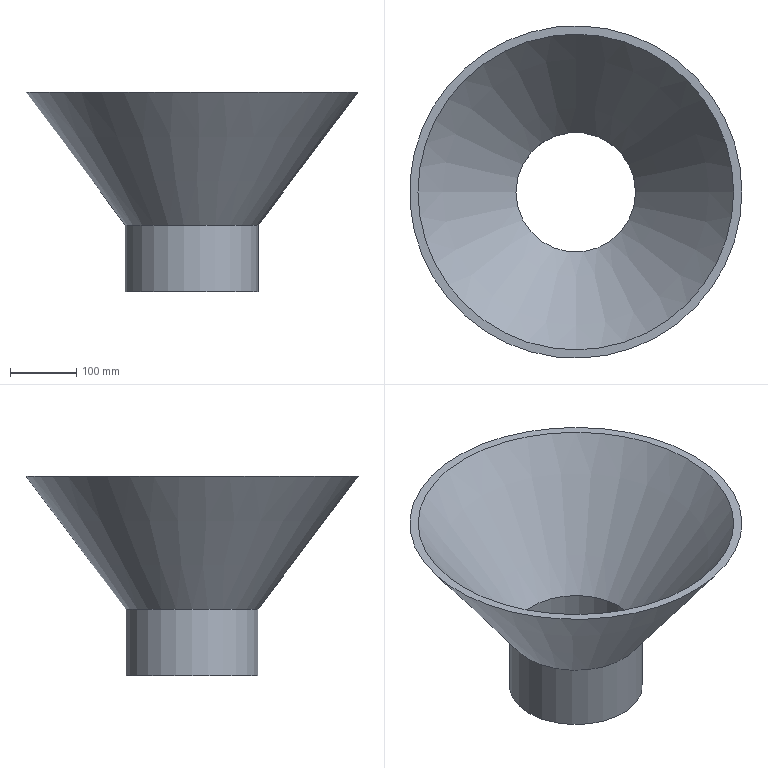Part | NX | features CONE 1, CYLINDER 1, DATUM_CSYS 1, SHELL 1 | 1 solid | 6 faces | box 500 x 500 x 300 mm | volume 3245287 mm3 | plane 2 | cylinder 2 | cone 2 | commonest cylinder face diameters 180 x1 200 x1
STEP:
#1=CARTESIAN_POINT('',(-90.,0.,0.));
#2=VERTEX_POINT('',#1);
#3=CARTESIAN_POINT('',(0.,0.,0.));
#4=DIRECTION('',(0.,0.,-1.));
#5=DIRECTION('',(-1.,0.,0.));
#6=AXIS2_PLACEMENT_3D('',#3,#4,#5);
#7=CIRCLE('',#6,90.);
#8=EDGE_CURVE('',#2,#2,#7,.F.);
#9=ORIENTED_EDGE('',*,*,#8,.T.);
#10=EDGE_LOOP('',(#9));
#11=FACE_BOUND('',#10,.T.);
#12=CARTESIAN_POINT('',(100.,0.,0.));
#13=VERTEX_POINT('',#12);
#14=CARTESIAN_POINT('',(0.,0.,0.));
#15=DIRECTION('',(0.,0.,1.));
#16=DIRECTION('',(1.,0.,0.));
#17=AXIS2_PLACEMENT_3D('',#14,#15,#16);
#18=CIRCLE('',#17,100.);
#19=EDGE_CURVE('',#13,#13,#18,.T.);
#20=ORIENTED_EDGE('',*,*,#19,.F.);
#21=EDGE_LOOP('',(#20));
#22=FACE_BOUND('',#21,.T.);
#23=CARTESIAN_POINT('',(0.,0.,0.));
#24=DIRECTION('',(0.,0.,-1.));
#25=DIRECTION('',(-1.,0.,0.));
#26=AXIS2_PLACEMENT_3D('',#23,#24,#25);
#27=PLANE('',#26);
#28=ADVANCED_FACE('',(#11,#22),#27,.T.);
#29=CARTESIAN_POINT('',(100.,0.,100.));
#30=VERTEX_POINT('',#29);
#31=CARTESIAN_POINT('',(0.,0.,100.));
#32=DIRECTION('',(0.,0.,1.));
#33=DIRECTION('',(1.,0.,0.));
#34=AXIS2_PLACEMENT_3D('',#31,#32,#33);
#35=CIRCLE('',#34,100.);
#36=EDGE_CURVE('',#30,#30,#35,.T.);
#37=ORIENTED_EDGE('',*,*,#36,.F.);
#38=EDGE_LOOP('',(#37));
#39=FACE_BOUND('',#38,.T.);
#40=ORIENTED_EDGE('',*,*,#19,.T.);
#41=EDGE_LOOP('',(#40));
#42=FACE_BOUND('',#41,.T.);
#43=CARTESIAN_POINT('',(0.,0.,0.));
#44=DIRECTION('',(0.,0.,1.));
#45=DIRECTION('',(1.,0.,0.));
#46=AXIS2_PLACEMENT_3D('',#43,#44,#45);
#47=CYLINDRICAL_SURFACE('',#46,100.);
#48=ADVANCED_FACE('',(#39,#42),#47,.T.);
#49=CARTESIAN_POINT('',(237.5,0.,300.));
#50=VERTEX_POINT('',#49);
#51=CARTESIAN_POINT('',(0.,0.,300.));
#52=DIRECTION('',(0.,0.,1.));
#53=DIRECTION('',(1.,0.,0.));
#54=AXIS2_PLACEMENT_3D('',#51,#52,#53);
#55=CIRCLE('',#54,237.5);
#56=EDGE_CURVE('',#50,#50,#55,.F.);
#57=ORIENTED_EDGE('',*,*,#56,.T.);
#58=EDGE_LOOP('',(#57));
#59=FACE_BOUND('',#58,.T.);
#60=CARTESIAN_POINT('',(250.,0.,300.));
#61=VERTEX_POINT('',#60);
#62=CARTESIAN_POINT('',(0.,0.,300.));
#63=DIRECTION('',(0.,0.,-1.));
#64=DIRECTION('',(1.,0.,0.));
#65=AXIS2_PLACEMENT_3D('',#62,#63,#64);
#66=CIRCLE('',#65,250.);
#67=EDGE_CURVE('',#61,#61,#66,.T.);
#68=ORIENTED_EDGE('',*,*,#67,.F.);
#69=EDGE_LOOP('',(#68));
#70=FACE_BOUND('',#69,.T.);
#71=CARTESIAN_POINT('',(0.,0.,300.));
#72=DIRECTION('',(0.,0.,1.));
#73=DIRECTION('',(1.,0.,0.));
#74=AXIS2_PLACEMENT_3D('',#71,#72,#73);
#75=PLANE('',#74);
#76=ADVANCED_FACE('',(#59,#70),#75,.T.);
#77=ORIENTED_EDGE('',*,*,#36,.T.);
#78=EDGE_LOOP('',(#77));
#79=FACE_BOUND('',#78,.T.);
#80=ORIENTED_EDGE('',*,*,#67,.T.);
#81=EDGE_LOOP('',(#80));
#82=FACE_BOUND('',#81,.T.);
#83=CARTESIAN_POINT('',(0.,0.,100.));
#84=DIRECTION('',(0.,0.,1.));
#85=DIRECTION('',(1.,0.,0.));
#86=AXIS2_PLACEMENT_3D('',#83,#84,#85);
#87=CONICAL_SURFACE('',#86,100.,0.6435);
#88=ADVANCED_FACE('',(#79,#82),#87,.T.);
#89=CARTESIAN_POINT('',(90.,0.,103.333));
#90=VERTEX_POINT('',#89);
#91=CARTESIAN_POINT('',(0.,0.,103.333));
#92=DIRECTION('',(0.,0.,1.));
#93=DIRECTION('',(1.,0.,0.));
#94=AXIS2_PLACEMENT_3D('',#91,#92,#93);
#95=CIRCLE('',#94,90.);
#96=EDGE_CURVE('',#90,#90,#95,.T.);
#97=ORIENTED_EDGE('',*,*,#96,.T.);
#98=EDGE_LOOP('',(#97));
#99=FACE_BOUND('',#98,.T.);
#100=ORIENTED_EDGE('',*,*,#8,.F.);
#101=EDGE_LOOP('',(#100));
#102=FACE_BOUND('',#101,.T.);
#103=CARTESIAN_POINT('',(0.,0.,0.));
#104=DIRECTION('',(0.,0.,1.));
#105=DIRECTION('',(1.,0.,0.));
#106=AXIS2_PLACEMENT_3D('',#103,#104,#105);
#107=CYLINDRICAL_SURFACE('',#106,90.);
#108=ADVANCED_FACE('',(#99,#102),#107,.F.);
#109=ORIENTED_EDGE('',*,*,#96,.F.);
#110=EDGE_LOOP('',(#109));
#111=FACE_BOUND('',#110,.T.);
#112=ORIENTED_EDGE('',*,*,#56,.F.);
#113=EDGE_LOOP('',(#112));
#114=FACE_BOUND('',#113,.T.);
#115=CARTESIAN_POINT('',(0.,0.,106.));
#116=DIRECTION('',(0.,0.,1.));
#117=DIRECTION('',(1.,0.,0.));
#118=AXIS2_PLACEMENT_3D('',#115,#116,#117);
#119=CONICAL_SURFACE('',#118,92.,0.6435);
#120=ADVANCED_FACE('',(#111,#114),#119,.F.);
#121=CLOSED_SHELL('',(#28,#48,#76,#88,#108,#120));
#122=MANIFOLD_SOLID_BREP('',#121);
#123=(LENGTH_UNIT()NAMED_UNIT(*)SI_UNIT(.MILLI.,.METRE.));
#124=UNCERTAINTY_MEASURE_WITH_UNIT(LENGTH_MEASURE(0.00001),#123,'','');
#125=(NAMED_UNIT(*)PLANE_ANGLE_UNIT()SI_UNIT($,.RADIAN.));
#126=(NAMED_UNIT(*)SI_UNIT($,.STERADIAN.)SOLID_ANGLE_UNIT());
#127=(GEOMETRIC_REPRESENTATION_CONTEXT(3)GLOBAL_UNCERTAINTY_ASSIGNED_CONTEXT((#124))GLOBAL_UNIT_ASSIGNED_CONTEXT((#123,#125,#126))REPRESENTATION_CONTEXT('',''));
#128=ADVANCED_BREP_SHAPE_REPRESENTATION('',(#122),#127);